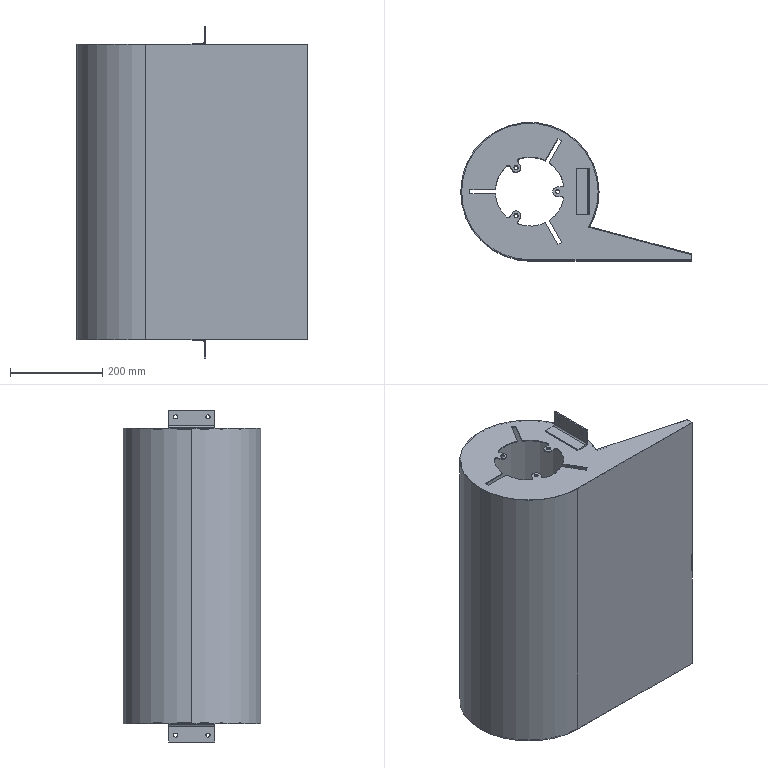Part | SolidWorks | features ICE 4, BaseBody 3 | 3 solids | 123 faces | box 500 x 300 x 720 mm | volume 2031659 mm3 | cylinder 67 | plane 56 | commonest cylinder face diameters 9 x20 10 x16 150 x12 20 x9 296 x3 300 x3